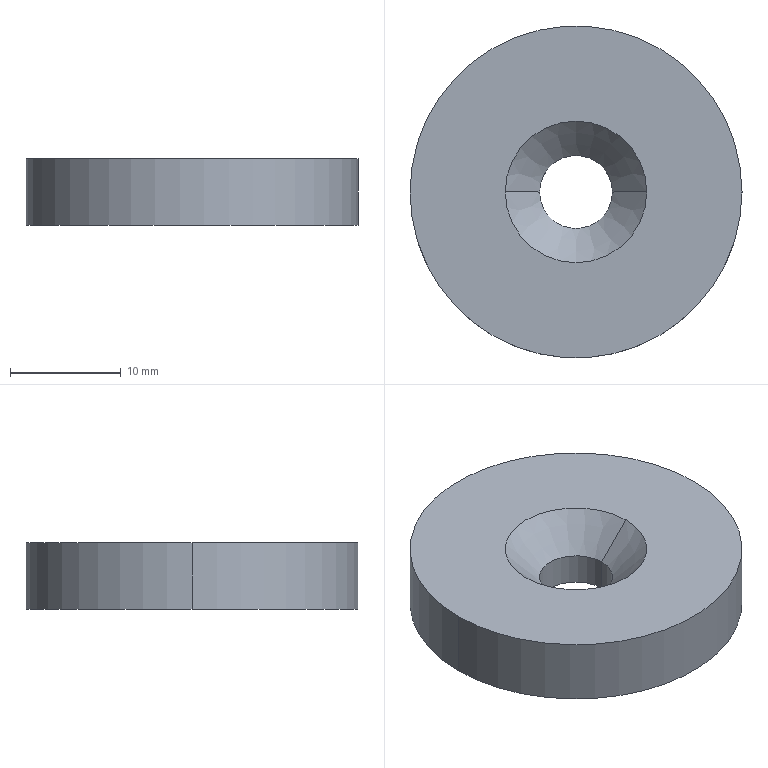Part | STEP file | 1 solid | 8 faces | box 30 x 30 x 6 mm | volume 3905 mm3 | cylinder 4 | cone 2 | plane 2 | commonest cylinder face diameters 6.6 x2 30 x2
STEP:
#1=CARTESIAN_POINT('',(0.,0.,0.));
#2=DIRECTION('',(0.,0.,1.));
#3=DIRECTION('',(1.,0.,0.));
#4=AXIS2_PLACEMENT_3D('',#1,#2,#3);
#5=CARTESIAN_POINT('',(-6.4,0.,6.));
#6=VERTEX_POINT('',#5);
#7=CARTESIAN_POINT('',(6.4,0.,6.));
#8=VERTEX_POINT('',#7);
#9=CARTESIAN_POINT('',(0.,0.,6.));
#10=DIRECTION('',(0.,0.,-1.));
#11=DIRECTION('',(1.,0.,0.));
#12=AXIS2_PLACEMENT_3D('',#9,#10,#11);
#13=CIRCLE('',#12,6.4);
#14=CARTESIAN_POINT('',(0.,0.,6.));
#15=DIRECTION('',(0.,0.,1.));
#16=DIRECTION('',(1.,0.,0.));
#17=AXIS2_PLACEMENT_3D('',#14,#15,#16);
#18=CONICAL_SURFACE('',#17,6.4,0.7854);
#19=CARTESIAN_POINT('',(6.283,0.));
#20=DIRECTION('',(-1.,0.));
#21=VECTOR('',#20,1.);
#22=LINE('',#19,#21);
#23=(GEOMETRIC_REPRESENTATION_CONTEXT(2)PARAMETRIC_REPRESENTATION_CONTEXT()REPRESENTATION_CONTEXT('',''));
#24=DEFINITIONAL_REPRESENTATION('',(#22),#23);
#25=PCURVE('',#18,#24);
#26=CARTESIAN_POINT('',(0.,0.,6.));
#27=DIRECTION('',(0.,0.,1.));
#28=DIRECTION('',(1.,0.,0.));
#29=AXIS2_PLACEMENT_3D('',#26,#27,#28);
#30=PLANE('',#29);
#31=CARTESIAN_POINT('',(6.4,0.));
#32=CARTESIAN_POINT('',(6.4,-11.085));
#33=CARTESIAN_POINT('',(-3.2,-5.543));
#34=CARTESIAN_POINT('',(-12.8,0.));
#35=CARTESIAN_POINT('',(-3.2,5.543));
#36=CARTESIAN_POINT('',(6.4,11.085));
#37=CARTESIAN_POINT('',(6.4,0.));
#38=(BOUNDED_CURVE()B_SPLINE_CURVE(2,(#31,#32,#33,#34,#35,#36,#37),.UNSPECIFIED.,.T.,.F.)B_SPLINE_CURVE_WITH_KNOTS((1,2,2,2,2,1),(-2.094,0.,2.094,4.189,6.283,8.378),.UNSPECIFIED.)CURVE()GEOMETRIC_REPRESENTATION_ITEM()RATIONAL_B_SPLINE_CURVE((1.,0.5,1.,0.5,1.,0.5,1.))REPRESENTATION_ITEM(''));
#39=(GEOMETRIC_REPRESENTATION_CONTEXT(2)PARAMETRIC_REPRESENTATION_CONTEXT()REPRESENTATION_CONTEXT('',''));
#40=DEFINITIONAL_REPRESENTATION('',(#38),#39);
#41=PCURVE('',#30,#40);
#42=SURFACE_CURVE('',#13,(#25,#41),.PCURVE_S1.);
#43=EDGE_CURVE('',#6,#8,#42,.T.);
#44=ORIENTED_EDGE('',*,*,#43,.T.);
#45=CARTESIAN_POINT('',(3.3,0.,2.9));
#46=VERTEX_POINT('',#45);
#47=CARTESIAN_POINT('',(6.4,0.,6.));
#48=DIRECTION('',(0.7071,0.,0.7071));
#49=VECTOR('',#48,1.);
#50=LINE('',#47,#49);
#51=CARTESIAN_POINT('',(0.,0.));
#52=DIRECTION('',(0.,1.));
#53=VECTOR('',#52,1.);
#54=LINE('',#51,#53);
#55=(GEOMETRIC_REPRESENTATION_CONTEXT(2)PARAMETRIC_REPRESENTATION_CONTEXT()REPRESENTATION_CONTEXT('',''));
#56=DEFINITIONAL_REPRESENTATION('',(#54),#55);
#57=PCURVE('',#18,#56);
#58=CARTESIAN_POINT('',(0.,0.,6.));
#59=DIRECTION('',(0.,0.,1.));
#60=DIRECTION('',(1.,0.,0.));
#61=AXIS2_PLACEMENT_3D('',#58,#59,#60);
#62=CONICAL_SURFACE('',#61,6.4,0.7854);
#63=CARTESIAN_POINT('',(6.283,0.));
#64=DIRECTION('',(0.,1.));
#65=VECTOR('',#64,1.);
#66=LINE('',#63,#65);
#67=(GEOMETRIC_REPRESENTATION_CONTEXT(2)PARAMETRIC_REPRESENTATION_CONTEXT()REPRESENTATION_CONTEXT('',''));
#68=DEFINITIONAL_REPRESENTATION('',(#66),#67);
#69=PCURVE('',#62,#68);
#70=SURFACE_CURVE('',#50,(#57,#69),.PCURVE_S1.);
#71=EDGE_CURVE('',#46,#8,#70,.T.);
#72=ORIENTED_EDGE('',*,*,#71,.F.);
#73=CARTESIAN_POINT('',(-3.3,0.,2.9));
#74=VERTEX_POINT('',#73);
#75=CARTESIAN_POINT('',(0.,0.,2.9));
#76=DIRECTION('',(0.,0.,-1.));
#77=DIRECTION('',(1.,0.,0.));
#78=AXIS2_PLACEMENT_3D('',#75,#76,#77);
#79=CIRCLE('',#78,3.3);
#80=CARTESIAN_POINT('',(6.283,-3.1));
#81=DIRECTION('',(-1.,0.));
#82=VECTOR('',#81,1.);
#83=LINE('',#80,#82);
#84=(GEOMETRIC_REPRESENTATION_CONTEXT(2)PARAMETRIC_REPRESENTATION_CONTEXT()REPRESENTATION_CONTEXT('',''));
#85=DEFINITIONAL_REPRESENTATION('',(#83),#84);
#86=PCURVE('',#18,#85);
#87=CARTESIAN_POINT('',(0.,0.,6.));
#88=DIRECTION('',(0.,0.,1.));
#89=DIRECTION('',(1.,0.,0.));
#90=AXIS2_PLACEMENT_3D('',#87,#88,#89);
#91=CYLINDRICAL_SURFACE('',#90,3.3);
#92=CARTESIAN_POINT('',(6.283,-3.1));
#93=DIRECTION('',(-1.,0.));
#94=VECTOR('',#93,1.);
#95=LINE('',#92,#94);
#96=(GEOMETRIC_REPRESENTATION_CONTEXT(2)PARAMETRIC_REPRESENTATION_CONTEXT()REPRESENTATION_CONTEXT('',''));
#97=DEFINITIONAL_REPRESENTATION('',(#95),#96);
#98=PCURVE('',#91,#97);
#99=SURFACE_CURVE('',#79,(#86,#98),.PCURVE_S1.);
#100=EDGE_CURVE('',#74,#46,#99,.T.);
#101=ORIENTED_EDGE('',*,*,#100,.F.);
#102=CARTESIAN_POINT('',(-6.4,0.,6.));
#103=DIRECTION('',(-0.7071,0.,0.7071));
#104=VECTOR('',#103,1.);
#105=LINE('',#102,#104);
#106=CARTESIAN_POINT('',(3.142,0.));
#107=DIRECTION('',(0.,1.));
#108=VECTOR('',#107,1.);
#109=LINE('',#106,#108);
#110=(GEOMETRIC_REPRESENTATION_CONTEXT(2)PARAMETRIC_REPRESENTATION_CONTEXT()REPRESENTATION_CONTEXT('',''));
#111=DEFINITIONAL_REPRESENTATION('',(#109),#110);
#112=PCURVE('',#18,#111);
#113=CARTESIAN_POINT('',(3.142,0.));
#114=DIRECTION('',(0.,1.));
#115=VECTOR('',#114,1.);
#116=LINE('',#113,#115);
#117=(GEOMETRIC_REPRESENTATION_CONTEXT(2)PARAMETRIC_REPRESENTATION_CONTEXT()REPRESENTATION_CONTEXT('',''));
#118=DEFINITIONAL_REPRESENTATION('',(#116),#117);
#119=PCURVE('',#62,#118);
#120=SURFACE_CURVE('',#105,(#112,#119),.PCURVE_S1.);
#121=EDGE_CURVE('',#74,#6,#120,.T.);
#122=ORIENTED_EDGE('',*,*,#121,.T.);
#123=EDGE_LOOP('',(#44,#72,#101,#122));
#124=FACE_BOUND('',#123,.F.);
#125=ADVANCED_FACE('',(#124),#18,.F.);
#126=CARTESIAN_POINT('',(0.,0.,6.));
#127=DIRECTION('',(0.,0.,-1.));
#128=DIRECTION('',(1.,0.,0.));
#129=AXIS2_PLACEMENT_3D('',#126,#127,#128);
#130=CIRCLE('',#129,6.4);
#131=CARTESIAN_POINT('',(6.4,0.));
#132=CARTESIAN_POINT('',(6.4,-11.085));
#133=CARTESIAN_POINT('',(-3.2,-5.543));
#134=CARTESIAN_POINT('',(-12.8,0.));
#135=CARTESIAN_POINT('',(-3.2,5.543));
#136=CARTESIAN_POINT('',(6.4,11.085));
#137=CARTESIAN_POINT('',(6.4,0.));
#138=(BOUNDED_CURVE()B_SPLINE_CURVE(2,(#131,#132,#133,#134,#135,#136,#137),.UNSPECIFIED.,.T.,.F.)B_SPLINE_CURVE_WITH_KNOTS((1,2,2,2,2,1),(-2.094,0.,2.094,4.189,6.283,8.378),.UNSPECIFIED.)CURVE()GEOMETRIC_REPRESENTATION_ITEM()RATIONAL_B_SPLINE_CURVE((1.,0.5,1.,0.5,1.,0.5,1.))REPRESENTATION_ITEM(''));
#139=(GEOMETRIC_REPRESENTATION_CONTEXT(2)PARAMETRIC_REPRESENTATION_CONTEXT()REPRESENTATION_CONTEXT('',''));
#140=DEFINITIONAL_REPRESENTATION('',(#138),#139);
#141=PCURVE('',#30,#140);
#142=CARTESIAN_POINT('',(6.283,0.));
#143=DIRECTION('',(-1.,0.));
#144=VECTOR('',#143,1.);
#145=LINE('',#142,#144);
#146=(GEOMETRIC_REPRESENTATION_CONTEXT(2)PARAMETRIC_REPRESENTATION_CONTEXT()REPRESENTATION_CONTEXT('',''));
#147=DEFINITIONAL_REPRESENTATION('',(#145),#146);
#148=PCURVE('',#62,#147);
#149=SURFACE_CURVE('',#130,(#141,#148),.PCURVE_S1.);
#150=EDGE_CURVE('',#8,#6,#149,.T.);
#151=ORIENTED_EDGE('',*,*,#150,.T.);
#152=ORIENTED_EDGE('',*,*,#43,.T.);
#153=EDGE_LOOP('',(#151,#152));
#154=FACE_BOUND('',#153,.T.);
#155=CARTESIAN_POINT('',(-15.,0.,6.));
#156=VERTEX_POINT('',#155);
#157=CARTESIAN_POINT('',(15.,0.,6.));
#158=VERTEX_POINT('',#157);
#159=CARTESIAN_POINT('',(0.,0.,6.));
#160=DIRECTION('',(0.,0.,-1.));
#161=DIRECTION('',(-1.,0.,0.));
#162=AXIS2_PLACEMENT_3D('',#159,#160,#161);
#163=CIRCLE('',#162,15.);
#164=CARTESIAN_POINT('',(-15.,0.));
#165=CARTESIAN_POINT('',(-15.,25.981));
#166=CARTESIAN_POINT('',(7.5,12.99));
#167=CARTESIAN_POINT('',(30.,0.));
#168=CARTESIAN_POINT('',(7.5,-12.99));
#169=CARTESIAN_POINT('',(-15.,-25.981));
#170=CARTESIAN_POINT('',(-15.,0.));
#171=(BOUNDED_CURVE()B_SPLINE_CURVE(2,(#164,#165,#166,#167,#168,#169,#170),.UNSPECIFIED.,.T.,.F.)B_SPLINE_CURVE_WITH_KNOTS((1,2,2,2,2,1),(-2.094,0.,2.094,4.189,6.283,8.378),.UNSPECIFIED.)CURVE()GEOMETRIC_REPRESENTATION_ITEM()RATIONAL_B_SPLINE_CURVE((1.,0.5,1.,0.5,1.,0.5,1.))REPRESENTATION_ITEM(''));
#172=(GEOMETRIC_REPRESENTATION_CONTEXT(2)PARAMETRIC_REPRESENTATION_CONTEXT()REPRESENTATION_CONTEXT('',''));
#173=DEFINITIONAL_REPRESENTATION('',(#171),#172);
#174=PCURVE('',#30,#173);
#175=CARTESIAN_POINT('',(0.,0.,6.));
#176=DIRECTION('',(0.,0.,-1.));
#177=DIRECTION('',(-1.,0.,0.));
#178=AXIS2_PLACEMENT_3D('',#175,#176,#177);
#179=CYLINDRICAL_SURFACE('',#178,15.);
#180=CARTESIAN_POINT('',(0.,0.));
#181=DIRECTION('',(1.,0.));
#182=VECTOR('',#181,1.);
#183=LINE('',#180,#182);
#184=(GEOMETRIC_REPRESENTATION_CONTEXT(2)PARAMETRIC_REPRESENTATION_CONTEXT()REPRESENTATION_CONTEXT('',''));
#185=DEFINITIONAL_REPRESENTATION('',(#183),#184);
#186=PCURVE('',#179,#185);
#187=SURFACE_CURVE('',#163,(#174,#186),.PCURVE_S1.);
#188=EDGE_CURVE('',#156,#158,#187,.T.);
#189=ORIENTED_EDGE('',*,*,#188,.F.);
#190=CARTESIAN_POINT('',(0.,0.,6.));
#191=DIRECTION('',(0.,0.,-1.));
#192=DIRECTION('',(-1.,0.,0.));
#193=AXIS2_PLACEMENT_3D('',#190,#191,#192);
#194=CIRCLE('',#193,15.);
#195=CARTESIAN_POINT('',(-15.,0.));
#196=CARTESIAN_POINT('',(-15.,25.981));
#197=CARTESIAN_POINT('',(7.5,12.99));
#198=CARTESIAN_POINT('',(30.,0.));
#199=CARTESIAN_POINT('',(7.5,-12.99));
#200=CARTESIAN_POINT('',(-15.,-25.981));
#201=CARTESIAN_POINT('',(-15.,0.));
#202=(BOUNDED_CURVE()B_SPLINE_CURVE(2,(#195,#196,#197,#198,#199,#200,#201),.UNSPECIFIED.,.T.,.F.)B_SPLINE_CURVE_WITH_KNOTS((1,2,2,2,2,1),(-2.094,0.,2.094,4.189,6.283,8.378),.UNSPECIFIED.)CURVE()GEOMETRIC_REPRESENTATION_ITEM()RATIONAL_B_SPLINE_CURVE((1.,0.5,1.,0.5,1.,0.5,1.))REPRESENTATION_ITEM(''));
#203=(GEOMETRIC_REPRESENTATION_CONTEXT(2)PARAMETRIC_REPRESENTATION_CONTEXT()REPRESENTATION_CONTEXT('',''));
#204=DEFINITIONAL_REPRESENTATION('',(#202),#203);
#205=PCURVE('',#30,#204);
#206=CARTESIAN_POINT('',(0.,0.,6.));
#207=DIRECTION('',(0.,0.,-1.));
#208=DIRECTION('',(-1.,0.,0.));
#209=AXIS2_PLACEMENT_3D('',#206,#207,#208);
#210=CYLINDRICAL_SURFACE('',#209,15.);
#211=CARTESIAN_POINT('',(0.,0.));
#212=DIRECTION('',(1.,0.));
#213=VECTOR('',#212,1.);
#214=LINE('',#211,#213);
#215=(GEOMETRIC_REPRESENTATION_CONTEXT(2)PARAMETRIC_REPRESENTATION_CONTEXT()REPRESENTATION_CONTEXT('',''));
#216=DEFINITIONAL_REPRESENTATION('',(#214),#215);
#217=PCURVE('',#210,#216);
#218=SURFACE_CURVE('',#194,(#205,#217),.PCURVE_S1.);
#219=EDGE_CURVE('',#158,#156,#218,.T.);
#220=ORIENTED_EDGE('',*,*,#219,.F.);
#221=EDGE_LOOP('',(#189,#220));
#222=FACE_BOUND('',#221,.T.);
#223=ADVANCED_FACE('',(#154,#222),#30,.T.);
#224=ORIENTED_EDGE('',*,*,#100,.T.);
#225=CARTESIAN_POINT('',(3.3,0.,0.));
#226=VERTEX_POINT('',#225);
#227=CARTESIAN_POINT('',(3.3,0.,6.));
#228=DIRECTION('',(0.,0.,1.));
#229=VECTOR('',#228,1.);
#230=LINE('',#227,#229);
#231=CARTESIAN_POINT('',(0.,0.));
#232=DIRECTION('',(0.,1.));
#233=VECTOR('',#232,1.);
#234=LINE('',#231,#233);
#235=(GEOMETRIC_REPRESENTATION_CONTEXT(2)PARAMETRIC_REPRESENTATION_CONTEXT()REPRESENTATION_CONTEXT('',''));
#236=DEFINITIONAL_REPRESENTATION('',(#234),#235);
#237=PCURVE('',#91,#236);
#238=CARTESIAN_POINT('',(0.,0.,6.));
#239=DIRECTION('',(0.,0.,1.));
#240=DIRECTION('',(1.,0.,0.));
#241=AXIS2_PLACEMENT_3D('',#238,#239,#240);
#242=CYLINDRICAL_SURFACE('',#241,3.3);
#243=CARTESIAN_POINT('',(6.283,0.));
#244=DIRECTION('',(0.,1.));
#245=VECTOR('',#244,1.);
#246=LINE('',#243,#245);
#247=(GEOMETRIC_REPRESENTATION_CONTEXT(2)PARAMETRIC_REPRESENTATION_CONTEXT()REPRESENTATION_CONTEXT('',''));
#248=DEFINITIONAL_REPRESENTATION('',(#246),#247);
#249=PCURVE('',#242,#248);
#250=SURFACE_CURVE('',#230,(#237,#249),.PCURVE_S1.);
#251=EDGE_CURVE('',#226,#46,#250,.T.);
#252=ORIENTED_EDGE('',*,*,#251,.F.);
#253=CARTESIAN_POINT('',(-3.3,0.,0.));
#254=VERTEX_POINT('',#253);
#255=CARTESIAN_POINT('',(0.,0.,0.));
#256=DIRECTION('',(0.,0.,-1.));
#257=DIRECTION('',(1.,0.,0.));
#258=AXIS2_PLACEMENT_3D('',#255,#256,#257);
#259=CIRCLE('',#258,3.3);
#260=CARTESIAN_POINT('',(6.283,-6.));
#261=DIRECTION('',(-1.,0.));
#262=VECTOR('',#261,1.);
#263=LINE('',#260,#262);
#264=(GEOMETRIC_REPRESENTATION_CONTEXT(2)PARAMETRIC_REPRESENTATION_CONTEXT()REPRESENTATION_CONTEXT('',''));
#265=DEFINITIONAL_REPRESENTATION('',(#263),#264);
#266=PCURVE('',#91,#265);
#267=CARTESIAN_POINT('',(0.,0.,0.));
#268=DIRECTION('',(0.,0.,1.));
#269=DIRECTION('',(1.,0.,0.));
#270=AXIS2_PLACEMENT_3D('',#267,#268,#269);
#271=PLANE('',#270);
#272=CARTESIAN_POINT('',(3.3,0.));
#273=CARTESIAN_POINT('',(3.3,-5.716));
#274=CARTESIAN_POINT('',(-1.65,-2.858));
#275=CARTESIAN_POINT('',(-6.6,0.));
#276=CARTESIAN_POINT('',(-1.65,2.858));
#277=CARTESIAN_POINT('',(3.3,5.716));
#278=CARTESIAN_POINT('',(3.3,0.));
#279=(BOUNDED_CURVE()B_SPLINE_CURVE(2,(#272,#273,#274,#275,#276,#277,#278),.UNSPECIFIED.,.T.,.F.)B_SPLINE_CURVE_WITH_KNOTS((1,2,2,2,2,1),(-2.094,0.,2.094,4.189,6.283,8.378),.UNSPECIFIED.)CURVE()GEOMETRIC_REPRESENTATION_ITEM()RATIONAL_B_SPLINE_CURVE((1.,0.5,1.,0.5,1.,0.5,1.))REPRESENTATION_ITEM(''));
#280=(GEOMETRIC_REPRESENTATION_CONTEXT(2)PARAMETRIC_REPRESENTATION_CONTEXT()REPRESENTATION_CONTEXT('',''));
#281=DEFINITIONAL_REPRESENTATION('',(#279),#280);
#282=PCURVE('',#271,#281);
#283=SURFACE_CURVE('',#259,(#266,#282),.PCURVE_S1.);
#284=EDGE_CURVE('',#254,#226,#283,.T.);
#285=ORIENTED_EDGE('',*,*,#284,.F.);
#286=CARTESIAN_POINT('',(-3.3,0.,6.));
#287=DIRECTION('',(0.,0.,1.));
#288=VECTOR('',#287,1.);
#289=LINE('',#286,#288);
#290=CARTESIAN_POINT('',(3.142,0.));
#291=DIRECTION('',(0.,1.));
#292=VECTOR('',#291,1.);
#293=LINE('',#290,#292);
#294=(GEOMETRIC_REPRESENTATION_CONTEXT(2)PARAMETRIC_REPRESENTATION_CONTEXT()REPRESENTATION_CONTEXT('',''));
#295=DEFINITIONAL_REPRESENTATION('',(#293),#294);
#296=PCURVE('',#91,#295);
#297=CARTESIAN_POINT('',(3.142,0.));
#298=DIRECTION('',(0.,1.));
#299=VECTOR('',#298,1.);
#300=LINE('',#297,#299);
#301=(GEOMETRIC_REPRESENTATION_CONTEXT(2)PARAMETRIC_REPRESENTATION_CONTEXT()REPRESENTATION_CONTEXT('',''));
#302=DEFINITIONAL_REPRESENTATION('',(#300),#301);
#303=PCURVE('',#242,#302);
#304=SURFACE_CURVE('',#289,(#296,#303),.PCURVE_S1.);
#305=EDGE_CURVE('',#254,#74,#304,.T.);
#306=ORIENTED_EDGE('',*,*,#305,.T.);
#307=EDGE_LOOP('',(#224,#252,#285,#306));
#308=FACE_BOUND('',#307,.F.);
#309=ADVANCED_FACE('',(#308),#91,.F.);
#310=CARTESIAN_POINT('',(15.,0.,0.));
#311=VERTEX_POINT('',#310);
#312=CARTESIAN_POINT('',(15.,0.,6.));
#313=DIRECTION('',(0.,0.,-1.));
#314=VECTOR('',#313,1.);
#315=LINE('',#312,#314);
#316=CARTESIAN_POINT('',(3.142,0.));
#317=DIRECTION('',(0.,1.));
#318=VECTOR('',#317,1.);
#319=LINE('',#316,#318);
#320=(GEOMETRIC_REPRESENTATION_CONTEXT(2)PARAMETRIC_REPRESENTATION_CONTEXT()REPRESENTATION_CONTEXT('',''));
#321=DEFINITIONAL_REPRESENTATION('',(#319),#320);
#322=PCURVE('',#210,#321);
#323=CARTESIAN_POINT('',(3.142,0.));
#324=DIRECTION('',(0.,1.));
#325=VECTOR('',#324,1.);
#326=LINE('',#323,#325);
#327=(GEOMETRIC_REPRESENTATION_CONTEXT(2)PARAMETRIC_REPRESENTATION_CONTEXT()REPRESENTATION_CONTEXT('',''));
#328=DEFINITIONAL_REPRESENTATION('',(#326),#327);
#329=PCURVE('',#179,#328);
#330=SURFACE_CURVE('',#315,(#322,#329),.PCURVE_S1.);
#331=EDGE_CURVE('',#158,#311,#330,.T.);
#332=ORIENTED_EDGE('',*,*,#331,.F.);
#333=ORIENTED_EDGE('',*,*,#219,.T.);
#334=CARTESIAN_POINT('',(-15.,0.,0.));
#335=VERTEX_POINT('',#334);
#336=CARTESIAN_POINT('',(-15.,0.,6.));
#337=DIRECTION('',(0.,0.,-1.));
#338=VECTOR('',#337,1.);
#339=LINE('',#336,#338);
#340=CARTESIAN_POINT('',(6.283,0.));
#341=DIRECTION('',(0.,1.));
#342=VECTOR('',#341,1.);
#343=LINE('',#340,#342);
#344=(GEOMETRIC_REPRESENTATION_CONTEXT(2)PARAMETRIC_REPRESENTATION_CONTEXT()REPRESENTATION_CONTEXT('',''));
#345=DEFINITIONAL_REPRESENTATION('',(#343),#344);
#346=PCURVE('',#210,#345);
#347=CARTESIAN_POINT('',(0.,0.));
#348=DIRECTION('',(0.,1.));
#349=VECTOR('',#348,1.);
#350=LINE('',#347,#349);
#351=(GEOMETRIC_REPRESENTATION_CONTEXT(2)PARAMETRIC_REPRESENTATION_CONTEXT()REPRESENTATION_CONTEXT('',''));
#352=DEFINITIONAL_REPRESENTATION('',(#350),#351);
#353=PCURVE('',#179,#352);
#354=SURFACE_CURVE('',#339,(#346,#353),.PCURVE_S1.);
#355=EDGE_CURVE('',#156,#335,#354,.T.);
#356=ORIENTED_EDGE('',*,*,#355,.T.);
#357=CARTESIAN_POINT('',(0.,0.,0.));
#358=DIRECTION('',(0.,0.,1.));
#359=DIRECTION('',(-1.,0.,0.));
#360=AXIS2_PLACEMENT_3D('',#357,#358,#359);
#361=CIRCLE('',#360,15.);
#362=CARTESIAN_POINT('',(6.283,6.));
#363=DIRECTION('',(-1.,0.));
#364=VECTOR('',#363,1.);
#365=LINE('',#362,#364);
#366=(GEOMETRIC_REPRESENTATION_CONTEXT(2)PARAMETRIC_REPRESENTATION_CONTEXT()REPRESENTATION_CONTEXT('',''));
#367=DEFINITIONAL_REPRESENTATION('',(#365),#366);
#368=PCURVE('',#210,#367);
#369=CARTESIAN_POINT('',(0.,0.));
#370=DIRECTION('',(-1.,0.));
#371=AXIS2_PLACEMENT_2D('',#369,#370);
#372=CIRCLE('',#371,15.);
#373=(GEOMETRIC_REPRESENTATION_CONTEXT(2)PARAMETRIC_REPRESENTATION_CONTEXT()REPRESENTATION_CONTEXT('',''));
#374=DEFINITIONAL_REPRESENTATION('',(#372),#373);
#375=PCURVE('',#271,#374);
#376=SURFACE_CURVE('',#361,(#368,#375),.PCURVE_S1.);
#377=EDGE_CURVE('',#335,#311,#376,.T.);
#378=ORIENTED_EDGE('',*,*,#377,.T.);
#379=EDGE_LOOP('',(#332,#333,#356,#378));
#380=FACE_BOUND('',#379,.T.);
#381=ADVANCED_FACE('',(#380),#210,.T.);
#382=CARTESIAN_POINT('',(0.,0.,0.));
#383=DIRECTION('',(0.,0.,-1.));
#384=DIRECTION('',(1.,0.,0.));
#385=AXIS2_PLACEMENT_3D('',#382,#383,#384);
#386=CIRCLE('',#385,3.3);
#387=CARTESIAN_POINT('',(3.3,0.));
#388=CARTESIAN_POINT('',(3.3,-5.716));
#389=CARTESIAN_POINT('',(-1.65,-2.858));
#390=CARTESIAN_POINT('',(-6.6,0.));
#391=CARTESIAN_POINT('',(-1.65,2.858));
#392=CARTESIAN_POINT('',(3.3,5.716));
#393=CARTESIAN_POINT('',(3.3,0.));
#394=(BOUNDED_CURVE()B_SPLINE_CURVE(2,(#387,#388,#389,#390,#391,#392,#393),.UNSPECIFIED.,.T.,.F.)B_SPLINE_CURVE_WITH_KNOTS((1,2,2,2,2,1),(-2.094,0.,2.094,4.189,6.283,8.378),.UNSPECIFIED.)CURVE()GEOMETRIC_REPRESENTATION_ITEM()RATIONAL_B_SPLINE_CURVE((1.,0.5,1.,0.5,1.,0.5,1.))REPRESENTATION_ITEM(''));
#395=(GEOMETRIC_REPRESENTATION_CONTEXT(2)PARAMETRIC_REPRESENTATION_CONTEXT()REPRESENTATION_CONTEXT('',''));
#396=DEFINITIONAL_REPRESENTATION('',(#394),#395);
#397=PCURVE('',#271,#396);
#398=CARTESIAN_POINT('',(6.283,-6.));
#399=DIRECTION('',(-1.,0.));
#400=VECTOR('',#399,1.);
#401=LINE('',#398,#400);
#402=(GEOMETRIC_REPRESENTATION_CONTEXT(2)PARAMETRIC_REPRESENTATION_CONTEXT()REPRESENTATION_CONTEXT('',''));
#403=DEFINITIONAL_REPRESENTATION('',(#401),#402);
#404=PCURVE('',#242,#403);
#405=SURFACE_CURVE('',#386,(#397,#404),.PCURVE_S1.);
#406=EDGE_CURVE('',#226,#254,#405,.T.);
#407=ORIENTED_EDGE('',*,*,#406,.F.);
#408=ORIENTED_EDGE('',*,*,#284,.F.);
#409=EDGE_LOOP('',(#407,#408));
#410=FACE_BOUND('',#409,.T.);
#411=ORIENTED_EDGE('',*,*,#377,.F.);
#412=CARTESIAN_POINT('',(0.,0.,0.));
#413=DIRECTION('',(0.,0.,1.));
#414=DIRECTION('',(-1.,0.,0.));
#415=AXIS2_PLACEMENT_3D('',#412,#413,#414);
#416=CIRCLE('',#415,15.);
#417=CARTESIAN_POINT('',(0.,0.));
#418=DIRECTION('',(-1.,0.));
#419=AXIS2_PLACEMENT_2D('',#417,#418);
#420=CIRCLE('',#419,15.);
#421=(GEOMETRIC_REPRESENTATION_CONTEXT(2)PARAMETRIC_REPRESENTATION_CONTEXT()REPRESENTATION_CONTEXT('',''));
#422=DEFINITIONAL_REPRESENTATION('',(#420),#421);
#423=PCURVE('',#271,#422);
#424=CARTESIAN_POINT('',(6.283,6.));
#425=DIRECTION('',(-1.,0.));
#426=VECTOR('',#425,1.);
#427=LINE('',#424,#426);
#428=(GEOMETRIC_REPRESENTATION_CONTEXT(2)PARAMETRIC_REPRESENTATION_CONTEXT()REPRESENTATION_CONTEXT('',''));
#429=DEFINITIONAL_REPRESENTATION('',(#427),#428);
#430=PCURVE('',#179,#429);
#431=SURFACE_CURVE('',#416,(#423,#430),.PCURVE_S1.);
#432=EDGE_CURVE('',#311,#335,#431,.T.);
#433=ORIENTED_EDGE('',*,*,#432,.F.);
#434=EDGE_LOOP('',(#411,#433));
#435=FACE_BOUND('',#434,.T.);
#436=ADVANCED_FACE('',(#410,#435),#271,.F.);
#437=ORIENTED_EDGE('',*,*,#71,.T.);
#438=ORIENTED_EDGE('',*,*,#150,.T.);
#439=ORIENTED_EDGE('',*,*,#121,.F.);
#440=CARTESIAN_POINT('',(0.,0.,2.9));
#441=DIRECTION('',(0.,0.,-1.));
#442=DIRECTION('',(1.,0.,0.));
#443=AXIS2_PLACEMENT_3D('',#440,#441,#442);
#444=CIRCLE('',#443,3.3);
#445=CARTESIAN_POINT('',(6.283,-3.1));
#446=DIRECTION('',(-1.,0.));
#447=VECTOR('',#446,1.);
#448=LINE('',#445,#447);
#449=(GEOMETRIC_REPRESENTATION_CONTEXT(2)PARAMETRIC_REPRESENTATION_CONTEXT()REPRESENTATION_CONTEXT('',''));
#450=DEFINITIONAL_REPRESENTATION('',(#448),#449);
#451=PCURVE('',#62,#450);
#452=CARTESIAN_POINT('',(6.283,-3.1));
#453=DIRECTION('',(-1.,0.));
#454=VECTOR('',#453,1.);
#455=LINE('',#452,#454);
#456=(GEOMETRIC_REPRESENTATION_CONTEXT(2)PARAMETRIC_REPRESENTATION_CONTEXT()REPRESENTATION_CONTEXT('',''));
#457=DEFINITIONAL_REPRESENTATION('',(#455),#456);
#458=PCURVE('',#242,#457);
#459=SURFACE_CURVE('',#444,(#451,#458),.PCURVE_S1.);
#460=EDGE_CURVE('',#46,#74,#459,.T.);
#461=ORIENTED_EDGE('',*,*,#460,.F.);
#462=EDGE_LOOP('',(#437,#438,#439,#461));
#463=FACE_BOUND('',#462,.F.);
#464=ADVANCED_FACE('',(#463),#62,.F.);
#465=ORIENTED_EDGE('',*,*,#251,.T.);
#466=ORIENTED_EDGE('',*,*,#460,.T.);
#467=ORIENTED_EDGE('',*,*,#305,.F.);
#468=ORIENTED_EDGE('',*,*,#406,.F.);
#469=EDGE_LOOP('',(#465,#466,#467,#468));
#470=FACE_BOUND('',#469,.F.);
#471=ADVANCED_FACE('',(#470),#242,.F.);
#472=ORIENTED_EDGE('',*,*,#188,.T.);
#473=ORIENTED_EDGE('',*,*,#331,.T.);
#474=ORIENTED_EDGE('',*,*,#432,.T.);
#475=ORIENTED_EDGE('',*,*,#355,.F.);
#476=EDGE_LOOP('',(#472,#473,#474,#475));
#477=FACE_BOUND('',#476,.T.);
#478=ADVANCED_FACE('',(#477),#179,.T.);
#479=CLOSED_SHELL('',(#125,#223,#309,#381,#436,#464,#471,#478));
#480=MANIFOLD_SOLID_BREP('',#479);
#481=(LENGTH_UNIT()NAMED_UNIT(*)SI_UNIT(.MILLI.,.METRE.));
#482=UNCERTAINTY_MEASURE_WITH_UNIT(LENGTH_MEASURE(0.0000001),#481,'','');
#483=(NAMED_UNIT(*)PLANE_ANGLE_UNIT()SI_UNIT($,.RADIAN.));
#484=(NAMED_UNIT(*)SI_UNIT($,.STERADIAN.)SOLID_ANGLE_UNIT());
#485=(GEOMETRIC_REPRESENTATION_CONTEXT(3)GLOBAL_UNCERTAINTY_ASSIGNED_CONTEXT((#482))GLOBAL_UNIT_ASSIGNED_CONTEXT((#481,#483,#484))REPRESENTATION_CONTEXT('',''));
#486=ADVANCED_BREP_SHAPE_REPRESENTATION('',(#4,#480),#485);